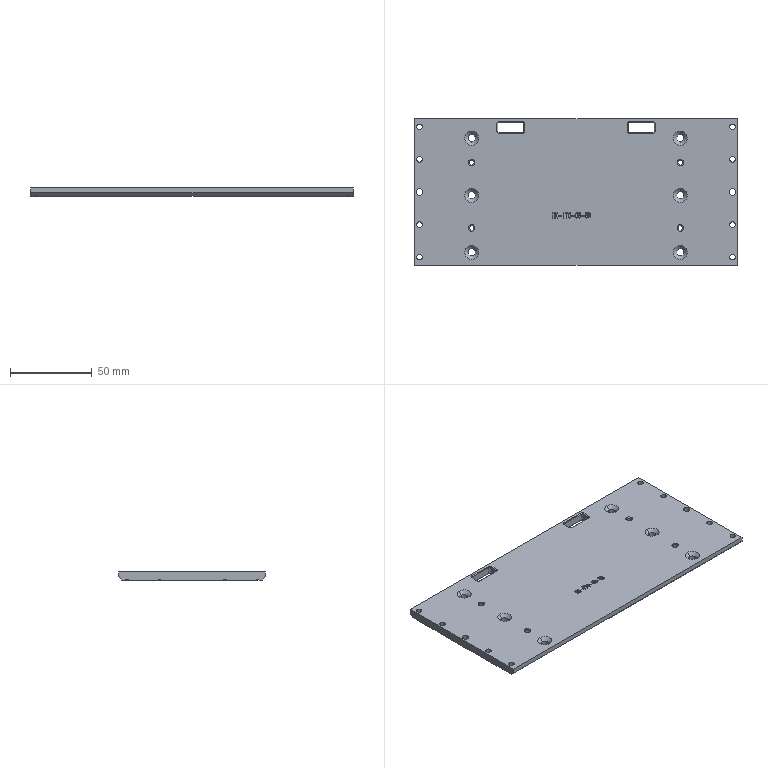NC program | NX | posted with a generic post | part box 198 x 90 x 5 mm
Lines 1 to 1351 of 7160:
N10 G17 G21 G94 G90
(DRILLING , TOOL : D6A45)
N12 T01 M6
N14 G54
N16 G17 G0 G90 X96. Y0. S5000 M3
N18 G43 Z30. H1
N20 G94 G81 G98 Z-2.5 F350. R3.
N22 X-96.
N24 G80
N26 G0 X-96. Y0. Z30.
(DRILLING_COPY , TOOL : D6A45)
N28 X-64. Y-22.
N30 G81 Z-2. F350. R3.
N32 Y18.
N34 X64. Y-22.
N36 Y18.
N38 G80
N40 G0 X64. Y18. Z30.
(DRILLING_COPY_COPY , TOOL : D6A45)
N42 X96. Y40.
N44 G81 Z-2.35 F350. R3.
N46 Y20.
N48 Y-20.
N50 Y-40.
N52 X64. Y-37.
N54 Y-2.
N56 Y33.
N58 X-64.
N60 Y-2.
N62 Y-37.
N64 X-96. Y-40.
N66 Y-20.
N68 Y20.
N70 Y40.
N72 G80
N74 G0 X-96. Y40. Z30.
N76 M5
(DRILLING_COPY_1 , TOOL : 4.5ZT)
N78 T08 M6
N80 G54
N82 G17 G0 G90 X-64. Y-37. S2000 M3
N84 G43 Z30. H8
N86 G94 G83 G98 Z-7.852 F300. Q2. R3.
N88 Y-2.
N90 Y33.
N92 X64.
N94 Y-2.
N96 Y-37.
N98 G80
N100 G0 X64. Y-37. Z30.
N102 M5
(DRILLING_COPY_1_COPY , TOOL : 3.4ZT)
N104 T16 M6
N106 G54
N108 G17 G0 G90 X-96. Y-40. S2000 M3
N110 G43 Z30. H16
N112 G94 G83 G98 Z-6.521 F200. Q2. R3.
N114 Y-20.
N116 Y20.
N118 Y40.
N120 X96.
N122 Y20.
N124 Y-20.
N126 Y-40.
N128 G80
N130 G0 X96. Y-40. Z30.
N132 M5
(ZLEVEL_PROFILE_COPY_1_COPY , TOOL : D10)
N134 T15 M6
N136 G54
N138 G17 G0 G90 X-104.1 Y13.918 S9500 M3
N140 G43 Z30. H15
N142 Z1.5
N144 G94 G1 Y45.554 Z-0.158 F1000.
N146 X-103.766 Y46.898 Z-0.231
N148 X-103.084 Y48.104 Z-0.303
N150 X-102.104 Y49.084 Z-0.376
N152 X-100.898 Y49.766 Z-0.448
N154 X-99.554 Y50.1 Z-0.521
N156 X-99. Z-0.55
N158 X99. F3000.
N160 G2 X104.1 Y45. R5.1
N162 G1 Y-45.
N164 G2 X99. Y-50.1 R5.1
N166 G1 X-99.
N168 G2 X-104.1 Y-45. R5.1
N170 G1 Y45.
N172 G2 X-99. Y50.1 R5.1
N174 G1 X99. Z-0.729
N176 X99.5 Y50.075 Z-0.73
N178 X99.995 Y50.002
N180 X100.48 Y49.88
N182 X100.952 Y49.712 Z-0.731
N184 X101.404 Y49.498
N186 X101.833 Y49.24 Z-0.732
N188 X102.235 Y48.942
N190 X102.606 Y48.606 Z-0.733
N192 X102.942 Y48.235
N194 X103.24 Y47.833 Z-0.734
N196 X103.498 Y47.404
N198 X103.712 Y46.952 Z-0.735
N200 X103.88 Y46.48
N202 X104.002 Y45.995
N204 X104.075 Y45.5 Z-0.736
N206 X104.1 Y45.
N208 X104.103 Y40. Z-0.741
N210 X104.1 Y35. Z-0.745
N212 Y-35. Z-0.809
N214 X104.103 Y-40. Z-0.813
N216 X104.1 Y-45. Z-0.818
N218 X104.075 Y-45.5
N220 X104.002 Y-45.995 Z-0.819
N222 X103.88 Y-46.48
N224 X103.712 Y-46.952 Z-0.82
N226 X103.498 Y-47.404
N228 X103.24 Y-47.833
N230 X102.942 Y-48.235 Z-0.821
N232 X102.606 Y-48.606
N234 X102.235 Y-48.942 Z-0.822
N236 X101.833 Y-49.24
N238 X101.404 Y-49.498 Z-0.823
N240 X100.952 Y-49.712
N242 X100.48 Y-49.88 Z-0.824
N244 X99.995 Y-50.002
N246 X99.5 Y-50.075 Z-0.825
N248 X99. Y-50.1
N250 X-99. Z-1.004
N252 X-99.5 Y-50.075 Z-1.005
N254 X-99.995 Y-50.002
N256 X-100.48 Y-49.88
N258 X-100.952 Y-49.712 Z-1.006
N260 X-101.404 Y-49.498
N262 X-101.833 Y-49.24 Z-1.007
N264 X-102.235 Y-48.942
N266 X-102.606 Y-48.606 Z-1.008
N268 X-102.942 Y-48.235
N270 X-103.24 Y-47.833 Z-1.009
N272 X-103.498 Y-47.404
N274 X-103.712 Y-46.952 Z-1.01
N276 X-103.88 Y-46.48
N278 X-104.002 Y-45.995
N280 X-104.075 Y-45.5 Z-1.011
N282 X-104.1 Y-45.
N284 X-104.103 Y-40. Z-1.016
N286 X-104.1 Y-35. Z-1.02
N288 Y35. Z-1.084
N290 X-104.103 Y40. Z-1.088
N292 X-104.1 Y45. Z-1.093
N294 X-104.075 Y45.5
N296 X-104.002 Y45.995 Z-1.094
N298 X-103.88 Y46.48
N300 X-103.712 Y46.952 Z-1.095
N302 X-103.498 Y47.404
N304 X-103.24 Y47.833
N306 X-102.942 Y48.235 Z-1.096
N308 X-102.606 Y48.606
N310 X-102.235 Y48.942 Z-1.097
N312 X-101.833 Y49.24
N314 X-101.404 Y49.498 Z-1.098
N316 X-100.952 Y49.712
N318 X-100.48 Y49.88 Z-1.099
N320 X-99.995 Y50.002
N322 X-99.5 Y50.075 Z-1.1
N324 X-99. Y50.1
N326 X99. Z-1.279
N328 X99.5 Y50.075 Z-1.28
N330 X99.995 Y50.002
N332 X100.48 Y49.88
N334 X100.952 Y49.712 Z-1.281
N336 X101.404 Y49.498
N338 X101.833 Y49.24 Z-1.282
N340 X102.235 Y48.942
N342 X102.606 Y48.606 Z-1.283
N344 X102.942 Y48.235
N346 X103.24 Y47.833 Z-1.284
N348 X103.498 Y47.404
N350 X103.712 Y46.952 Z-1.285
N352 X103.88 Y46.48
N354 X104.002 Y45.995
N356 X104.075 Y45.5 Z-1.286
N358 X104.1 Y45.
N360 X104.103 Y40. Z-1.291
N362 X104.1 Y35. Z-1.295
N364 Y-35. Z-1.359
N366 X104.103 Y-40. Z-1.363
N368 X104.1 Y-45. Z-1.368
N370 X104.075 Y-45.5
N372 X104.002 Y-45.995 Z-1.369
N374 X103.88 Y-46.48
N376 X103.712 Y-46.952 Z-1.37
N378 X103.498 Y-47.404
N380 X103.24 Y-47.833
N382 X102.942 Y-48.235 Z-1.371
N384 X102.606 Y-48.606
N386 X102.235 Y-48.942 Z-1.372
N388 X101.833 Y-49.24
N390 X101.404 Y-49.498 Z-1.373
N392 X100.952 Y-49.712
N394 X100.48 Y-49.88 Z-1.374
N396 X99.995 Y-50.002
N398 X99.5 Y-50.075 Z-1.375
N400 X99. Y-50.1
N402 X-99. Z-1.554
N404 X-99.5 Y-50.075 Z-1.555
N406 X-99.995 Y-50.002
N408 X-100.48 Y-49.88
N410 X-100.952 Y-49.712 Z-1.556
N412 X-101.404 Y-49.498
N414 X-101.833 Y-49.24 Z-1.557
N416 X-102.235 Y-48.942
N418 X-102.606 Y-48.606 Z-1.558
N420 X-102.942 Y-48.235
N422 X-103.24 Y-47.833 Z-1.559
N424 X-103.498 Y-47.404
N426 X-103.712 Y-46.952 Z-1.56
N428 X-103.88 Y-46.48
N430 X-104.002 Y-45.995
N432 X-104.075 Y-45.5 Z-1.561
N434 X-104.1 Y-45.
N436 X-104.103 Y-40. Z-1.566
N438 X-104.1 Y-35. Z-1.57
N440 Y35. Z-1.634
N442 X-104.103 Y40. Z-1.638
N444 X-104.1 Y45. Z-1.643
N446 X-104.075 Y45.5
N448 X-104.002 Y45.995 Z-1.644
N450 X-103.88 Y46.48
N452 X-103.712 Y46.952 Z-1.645
N454 X-103.498 Y47.404
N456 X-103.24 Y47.833
N458 X-102.942 Y48.235 Z-1.646
N460 X-102.606 Y48.606
N462 X-102.235 Y48.942 Z-1.647
N464 X-101.833 Y49.24
N466 X-101.404 Y49.498 Z-1.648
N468 X-100.952 Y49.712
N470 X-100.48 Y49.88 Z-1.649
N472 X-99.995 Y50.002
N474 X-99.5 Y50.075 Z-1.65
N476 X-99. Y50.1
N478 X99. Z-1.829
N480 X99.5 Y50.075 Z-1.83
N482 X99.995 Y50.002
N484 X100.48 Y49.88
N486 X100.952 Y49.712 Z-1.831
N488 X101.404 Y49.498
N490 X101.833 Y49.24 Z-1.832
N492 X102.235 Y48.942
N494 X102.606 Y48.606 Z-1.833
N496 X102.942 Y48.235
N498 X103.24 Y47.833 Z-1.834
N500 X103.498 Y47.404
N502 X103.712 Y46.952 Z-1.835
N504 X103.88 Y46.48
N506 X104.002 Y45.995
N508 X104.075 Y45.5 Z-1.836
N510 X104.1 Y45.
N512 X104.103 Y40. Z-1.841
N514 X104.1 Y35. Z-1.845
N516 Y-35. Z-1.909
N518 X104.103 Y-40. Z-1.913
N520 X104.1 Y-45. Z-1.918
N522 X104.075 Y-45.5
N524 X104.002 Y-45.995 Z-1.919
N526 X103.88 Y-46.48
N528 X103.712 Y-46.952 Z-1.92
N530 X103.498 Y-47.404
N532 X103.24 Y-47.833
N534 X102.942 Y-48.235 Z-1.921
N536 X102.606 Y-48.606
N538 X102.235 Y-48.942 Z-1.922
N540 X101.833 Y-49.24
N542 X101.404 Y-49.498 Z-1.923
N544 X100.952 Y-49.712
N546 X100.48 Y-49.88 Z-1.924
N548 X99.995 Y-50.002
N550 X99.5 Y-50.075 Z-1.925
N552 X99. Y-50.1
N554 X-99. Z-2.104
N556 X-99.5 Y-50.075 Z-2.105
N558 X-99.995 Y-50.002
N560 X-100.48 Y-49.88
N562 X-100.952 Y-49.712 Z-2.106
N564 X-101.404 Y-49.498
N566 X-101.833 Y-49.24 Z-2.107
N568 X-102.235 Y-48.942
N570 X-102.606 Y-48.606 Z-2.108
N572 X-102.942 Y-48.235
N574 X-103.24 Y-47.833 Z-2.109
N576 X-103.498 Y-47.404
N578 X-103.712 Y-46.952 Z-2.11
N580 X-103.88 Y-46.48
N582 X-104.002 Y-45.995
N584 X-104.075 Y-45.5 Z-2.111
N586 X-104.1 Y-45.
N588 X-104.103 Y-40. Z-2.116
N590 X-104.1 Y-35. Z-2.12
N592 Y35. Z-2.184
N594 X-104.103 Y40. Z-2.188
N596 X-104.1 Y45. Z-2.193
N598 X-104.075 Y45.5
N600 X-104.002 Y45.995 Z-2.194
N602 X-103.88 Y46.48
N604 X-103.712 Y46.952 Z-2.195
N606 X-103.498 Y47.404
N608 X-103.24 Y47.833
N610 X-102.942 Y48.235 Z-2.196
N612 X-102.606 Y48.606
N614 X-102.235 Y48.942 Z-2.197
N616 X-101.833 Y49.24
N618 X-101.404 Y49.498 Z-2.198
N620 X-100.952 Y49.712
N622 X-100.48 Y49.88 Z-2.199
N624 X-99.995 Y50.002
N626 X-99.5 Y50.075 Z-2.2
N628 X-99. Y50.1
N630 X99. Z-2.379
N632 X99.5 Y50.075 Z-2.38
N634 X99.995 Y50.002
N636 X100.48 Y49.88
N638 X100.952 Y49.712 Z-2.381
N640 X101.404 Y49.498
N642 X101.833 Y49.24 Z-2.382
N644 X102.235 Y48.942
N646 X102.606 Y48.606 Z-2.383
N648 X102.942 Y48.235
N650 X103.24 Y47.833 Z-2.384
N652 X103.498 Y47.404
N654 X103.712 Y46.952 Z-2.385
N656 X103.88 Y46.48
N658 X104.002 Y45.995
N660 X104.075 Y45.5 Z-2.386
N662 X104.1 Y45.
N664 X104.103 Y40. Z-2.391
N666 X104.1 Y35. Z-2.395
N668 Y-35. Z-2.459
N670 X104.103 Y-40. Z-2.463
N672 X104.1 Y-45. Z-2.468
N674 X104.075 Y-45.5
N676 X104.002 Y-45.995 Z-2.469
N678 X103.88 Y-46.48
N680 X103.712 Y-46.952 Z-2.47
N682 X103.498 Y-47.404
N684 X103.24 Y-47.833
N686 X102.942 Y-48.235 Z-2.471
N688 X102.606 Y-48.606
N690 X102.235 Y-48.942 Z-2.472
N692 X101.833 Y-49.24
N694 X101.404 Y-49.498 Z-2.473
N696 X100.952 Y-49.712
N698 X100.48 Y-49.88 Z-2.474
N700 X99.995 Y-50.002
N702 X99.5 Y-50.075 Z-2.475
N704 X99. Y-50.1
N706 X-99. Z-2.654
N708 X-99.5 Y-50.075 Z-2.655
N710 X-99.995 Y-50.002
N712 X-100.48 Y-49.88
N714 X-100.952 Y-49.712 Z-2.656
N716 X-101.404 Y-49.498
N718 X-101.833 Y-49.24 Z-2.657
N720 X-102.235 Y-48.942
N722 X-102.606 Y-48.606 Z-2.658
N724 X-102.942 Y-48.235
N726 X-103.24 Y-47.833 Z-2.659
N728 X-103.498 Y-47.404
N730 X-103.712 Y-46.952 Z-2.66
N732 X-103.88 Y-46.48
N734 X-104.002 Y-45.995
N736 X-104.075 Y-45.5 Z-2.661
N738 X-104.1 Y-45.
N740 X-104.103 Y-40. Z-2.666
N742 X-104.1 Y-35. Z-2.67
N744 Y35. Z-2.734
N746 X-104.103 Y40. Z-2.738
N748 X-104.1 Y45. Z-2.743
N750 X-104.075 Y45.5
N752 X-104.002 Y45.995 Z-2.744
N754 X-103.88 Y46.48
N756 X-103.712 Y46.952 Z-2.745
N758 X-103.498 Y47.404
N760 X-103.24 Y47.833
N762 X-102.942 Y48.235 Z-2.746
N764 X-102.606 Y48.606
N766 X-102.235 Y48.942 Z-2.747
N768 X-101.833 Y49.24
N770 X-101.404 Y49.498 Z-2.748
N772 X-100.952 Y49.712
N774 X-100.48 Y49.88 Z-2.749
N776 X-99.995 Y50.002
N778 X-99.5 Y50.075 Z-2.75
N780 X-99. Y50.1
N782 X99. Z-2.929
N784 X99.5 Y50.075 Z-2.93
N786 X99.995 Y50.002
N788 X100.48 Y49.88
N790 X100.952 Y49.712 Z-2.931
N792 X101.404 Y49.498
N794 X101.833 Y49.24 Z-2.932
N796 X102.235 Y48.942
N798 X102.606 Y48.606 Z-2.933
N800 X102.942 Y48.235
N802 X103.24 Y47.833 Z-2.934
N804 X103.498 Y47.404
N806 X103.712 Y46.952 Z-2.935
N808 X103.88 Y46.48
N810 X104.002 Y45.995
N812 X104.075 Y45.5 Z-2.936
N814 X104.1 Y45.
N816 X104.103 Y40. Z-2.941
N818 X104.1 Y35. Z-2.945
N820 Y-35. Z-3.009
N822 X104.103 Y-40. Z-3.013
N824 X104.1 Y-45. Z-3.018
N826 X104.075 Y-45.5
N828 X104.002 Y-45.995 Z-3.019
N830 X103.88 Y-46.48
N832 X103.712 Y-46.952 Z-3.02
N834 X103.498 Y-47.404
N836 X103.24 Y-47.833
N838 X102.942 Y-48.235 Z-3.021
N840 X102.606 Y-48.606
N842 X102.235 Y-48.942 Z-3.022
N844 X101.833 Y-49.24
N846 X101.404 Y-49.498 Z-3.023
N848 X100.952 Y-49.712
N850 X100.48 Y-49.88 Z-3.024
N852 X99.995 Y-50.002
N854 X99.5 Y-50.075 Z-3.025
N856 X99. Y-50.1
N858 X-99. Z-3.204
N860 X-99.5 Y-50.075 Z-3.205
N862 X-99.995 Y-50.002
N864 X-100.48 Y-49.88
N866 X-100.952 Y-49.712 Z-3.206
N868 X-101.404 Y-49.498
N870 X-101.833 Y-49.24 Z-3.207
N872 X-102.235 Y-48.942
N874 X-102.606 Y-48.606 Z-3.208
N876 X-102.942 Y-48.235
N878 X-103.24 Y-47.833 Z-3.209
N880 X-103.498 Y-47.404
N882 X-103.712 Y-46.952 Z-3.21
N884 X-103.88 Y-46.48
N886 X-104.002 Y-45.995
N888 X-104.075 Y-45.5 Z-3.211
N890 X-104.1 Y-45.
N892 X-104.103 Y-40. Z-3.216
N894 X-104.1 Y-35. Z-3.22
N896 Y35. Z-3.284
N898 X-104.103 Y40. Z-3.288
N900 X-104.1 Y45. Z-3.293
N902 X-104.075 Y45.5
N904 X-104.002 Y45.995 Z-3.294
N906 X-103.88 Y46.48
N908 X-103.712 Y46.952 Z-3.295
N910 X-103.498 Y47.404
N912 X-103.24 Y47.833
N914 X-102.942 Y48.235 Z-3.296
N916 X-102.606 Y48.606
N918 X-102.235 Y48.942 Z-3.297
N920 X-101.833 Y49.24
N922 X-101.404 Y49.498 Z-3.298
N924 X-100.952 Y49.712
N926 X-100.48 Y49.88 Z-3.299
N928 X-99.995 Y50.002
N930 X-99.5 Y50.075 Z-3.3
N932 X-99. Y50.1
N934 X99. Z-3.479
N936 X99.5 Y50.075 Z-3.48
N938 X99.995 Y50.002
N940 X100.48 Y49.88
N942 X100.952 Y49.712 Z-3.481
N944 X101.404 Y49.498
N946 X101.833 Y49.24 Z-3.482
N948 X102.235 Y48.942
N950 X102.606 Y48.606 Z-3.483
N952 X102.942 Y48.235
N954 X103.24 Y47.833 Z-3.484
N956 X103.498 Y47.404
N958 X103.712 Y46.952 Z-3.485
N960 X103.88 Y46.48
N962 X104.002 Y45.995
N964 X104.075 Y45.5 Z-3.486
N966 X104.1 Y45.
N968 X104.103 Y40. Z-3.491
N970 X104.1 Y35. Z-3.495
N972 Y-35. Z-3.559
N974 X104.103 Y-40. Z-3.563
N976 X104.1 Y-45. Z-3.568
N978 X104.075 Y-45.5
N980 X104.002 Y-45.995 Z-3.569
N982 X103.88 Y-46.48
N984 X103.712 Y-46.952 Z-3.57
N986 X103.498 Y-47.404
N988 X103.24 Y-47.833
N990 X102.942 Y-48.235 Z-3.571
N992 X102.606 Y-48.606
N994 X102.235 Y-48.942 Z-3.572
N996 X101.833 Y-49.24
N998 X101.404 Y-49.498 Z-3.573
N1000 X100.952 Y-49.712
N1002 X100.48 Y-49.88 Z-3.574
N1004 X99.995 Y-50.002
N1006 X99.5 Y-50.075 Z-3.575
N1008 X99. Y-50.1
N1010 X-99. Z-3.754
N1012 X-99.5 Y-50.075 Z-3.755
N1014 X-99.995 Y-50.002
N1016 X-100.48 Y-49.88
N1018 X-100.952 Y-49.712 Z-3.756
N1020 X-101.404 Y-49.498
N1022 X-101.833 Y-49.24 Z-3.757
N1024 X-102.235 Y-48.942
N1026 X-102.606 Y-48.606 Z-3.758
N1028 X-102.942 Y-48.235
N1030 X-103.24 Y-47.833 Z-3.759
N1032 X-103.498 Y-47.404
N1034 X-103.712 Y-46.952 Z-3.76
N1036 X-103.88 Y-46.48
N1038 X-104.002 Y-45.995
N1040 X-104.075 Y-45.5 Z-3.761
N1042 X-104.1 Y-45.
N1044 X-104.103 Y-40. Z-3.766
N1046 X-104.1 Y-35. Z-3.77
N1048 Y35. Z-3.834
N1050 X-104.103 Y40. Z-3.838
N1052 X-104.1 Y45. Z-3.843
N1054 X-104.075 Y45.5
N1056 X-104.002 Y45.995 Z-3.844
N1058 X-103.88 Y46.48
N1060 X-103.712 Y46.952 Z-3.845
N1062 X-103.498 Y47.404
N1064 X-103.24 Y47.833
N1066 X-102.942 Y48.235 Z-3.846
N1068 X-102.606 Y48.606
N1070 X-102.235 Y48.942 Z-3.847
N1072 X-101.833 Y49.24
N1074 X-101.404 Y49.498 Z-3.848
N1076 X-100.952 Y49.712
N1078 X-100.48 Y49.88 Z-3.849
N1080 X-99.995 Y50.002
N1082 X-99.5 Y50.075 Z-3.85
N1084 X-99. Y50.1
N1086 X99. Z-4.029
N1088 X99.5 Y50.075 Z-4.03
N1090 X99.995 Y50.002
N1092 X100.48 Y49.88
N1094 X100.952 Y49.712 Z-4.031
N1096 X101.404 Y49.498
N1098 X101.833 Y49.24 Z-4.032
N1100 X102.235 Y48.942
N1102 X102.606 Y48.606 Z-4.033
N1104 X102.942 Y48.235
N1106 X103.24 Y47.833 Z-4.034
N1108 X103.498 Y47.404
N1110 X103.712 Y46.952 Z-4.035
N1112 X103.88 Y46.48
N1114 X104.002 Y45.995
N1116 X104.075 Y45.5 Z-4.036
N1118 X104.1 Y45.
N1120 X104.103 Y40. Z-4.041
N1122 X104.1 Y35. Z-4.045
N1124 Y-35. Z-4.109
N1126 X104.103 Y-40. Z-4.113
N1128 X104.1 Y-45. Z-4.118
N1130 X104.075 Y-45.5
N1132 X104.002 Y-45.995 Z-4.119
N1134 X103.88 Y-46.48
N1136 X103.712 Y-46.952 Z-4.12
N1138 X103.498 Y-47.404
N1140 X103.24 Y-47.833
N1142 X102.942 Y-48.235 Z-4.121
N1144 X102.606 Y-48.606
N1146 X102.235 Y-48.942 Z-4.122
N1148 X101.833 Y-49.24
N1150 X101.404 Y-49.498 Z-4.123
N1152 X100.952 Y-49.712
N1154 X100.48 Y-49.88 Z-4.124
N1156 X99.995 Y-50.002
N1158 X99.5 Y-50.075 Z-4.125
N1160 X99. Y-50.1
N1162 X-99. Z-4.304
N1164 X-99.5 Y-50.075 Z-4.305
N1166 X-99.995 Y-50.002
N1168 X-100.48 Y-49.88
N1170 X-100.952 Y-49.712 Z-4.306
N1172 X-101.404 Y-49.498
N1174 X-101.833 Y-49.24 Z-4.307
N1176 X-102.235 Y-48.942
N1178 X-102.606 Y-48.606 Z-4.308
N1180 X-102.942 Y-48.235
N1182 X-103.24 Y-47.833 Z-4.309
N1184 X-103.498 Y-47.404
N1186 X-103.712 Y-46.952 Z-4.31
N1188 X-103.88 Y-46.48
N1190 X-104.002 Y-45.995
N1192 X-104.075 Y-45.5 Z-4.311
N1194 X-104.1 Y-45.
N1196 X-104.103 Y-40. Z-4.316
N1198 X-104.1 Y-35. Z-4.32
N1200 Y35. Z-4.384
N1202 X-104.103 Y40. Z-4.388
N1204 X-104.1 Y45. Z-4.393
N1206 X-104.075 Y45.5
N1208 X-104.002 Y45.995 Z-4.394
N1210 X-103.88 Y46.48
N1212 X-103.712 Y46.952 Z-4.395
N1214 X-103.498 Y47.404
N1216 X-103.24 Y47.833
N1218 X-102.942 Y48.235 Z-4.396
N1220 X-102.606 Y48.606
N1222 X-102.235 Y48.942 Z-4.397
N1224 X-101.833 Y49.24
N1226 X-101.404 Y49.498 Z-4.398
N1228 X-100.952 Y49.712
N1230 X-100.48 Y49.88 Z-4.399
N1232 X-99.995 Y50.002
N1234 X-99.5 Y50.075 Z-4.4
N1236 X-99. Y50.1
N1238 X99.
N1240 G2 X104.1 Y45. R5.1
N1242 G1 Y-45.
N1244 G2 X99. Y-50.1 R5.1
N1246 G1 X-99.
N1248 G2 X-104.1 Y-45. R5.1
N1250 G1 Y45.
N1252 G2 X-99. Y50.1 R5.1
N1254 G1 Z-2.9
N1256 G0 Z30.
(FLOOR_WALL , TOOL : D10)
N1258 X75.1 Y-14.822
N1260 Z1.5
N1262 G1 Y-26.5 Z0.888 F1000.
N1264 Y-26.734 Z0.876
N1266 X75.342 Y-27.158 Z0.85
N1268 X75.766 Y-27.4 Z0.825
N1270 X82.234 Z0.486
N1272 X82.658 Y-27.158 Z0.46
N1274 X82.9 Y-26.734 Z0.434
N1276 Y-26.5 Z0.422
N1278 Y0. Z-0.967
N1280 Y26.5 F3000.
N1282 G3 X82. Y27.4 R0.9
N1284 G1 X76.
N1286 G3 X75.1 Y26.5 R0.9
N1288 G1 Y-26.5
N1290 G3 X76. Y-27.4 R0.9
N1292 G1 X82.
N1294 G3 X82.9 Y-26.5 R0.9
N1296 G1 Y0.
N1298 Z0.533
N1300 G0 X75.1 Y-14.822
N1302 G1 Y-26.5 Z-0.079 F1000.
N1304 Y-26.734 Z-0.091
N1306 X75.342 Y-27.158 Z-0.117
N1308 X75.766 Y-27.4 Z-0.142
N1310 X82.234 Z-0.481
N1312 X82.658 Y-27.158 Z-0.507
N1314 X82.9 Y-26.734 Z-0.532
N1316 Y-26.5 Z-0.545
N1318 Y0. Z-1.933
N1320 Y26.5 F3000.
N1322 G3 X82. Y27.4 R0.9
N1324 G1 X76.
N1326 G3 X75.1 Y26.5 R0.9
N1328 G1 Y-26.5
N1330 G3 X76. Y-27.4 R0.9
N1332 G1 X82.
N1334 G3 X82.9 Y-26.5 R0.9
N1336 G1 Y0.
N1338 Z-0.433
N1340 G0 X75.1 Y-14.822
N1342 G1 Y-26.5 Z-1.045 F1000.
N1344 Y-26.734 Z-1.058
N1346 X75.342 Y-27.158 Z-1.083
N1348 X75.766 Y-27.4 Z-1.109
N1350 X82.234 Z-1.448
N1352 X82.658 Y-27.158 Z-1.473
N1354 X82.9 Y-26.734 Z-1.499
N1356 Y-26.5 Z-1.511
N1358 Y0. Z-2.9
N1360 Y26.5 F3000.
N1362 G3 X82. Y27.4 R0.9
N1364 G1 X76.
N1366 G3 X75.1 Y26.5 R0.9
N1368 G1 Y-26.5
N1370 G3 X76. Y-27.4 R0.9
N1372 G1 X82.
N1374 G3 X82.9 Y-26.5 R0.9
N1376 G1 Y0.
N1378 Z-1.4
N1380 G0 Z30.
N1382 X-31.9 Y0.267
N1384 Z1.5
N1386 G1 Y-6.4 Z1.151 F1000.
N1388 X-29.1 Z1.004
N1390 Y6.4 Z0.333
N1392 X-31.9 Z0.186
N1394 Y-6.4 Z-0.485
N1396 X-29.1 Z-0.631
N1398 Y0. Z-0.967
N1400 Y6.4 F3000.
N1402 X-31.9
N1404 Y-6.4
N1406 X-29.1
N1408 Y0.
N1410 X-22.1
N1412 Y13.4
N1414 X-38.9
N1416 Y-13.4
N1418 X-22.1
N1420 Y0.
N1422 X-15.1
N1424 Y20.4
N1426 X-45.9
N1428 Y-20.4
N1430 X-15.1
N1432 Y0.
N1434 X-8.1
N1436 Y26.5
N1438 G3 X-9. Y27.4 R0.9
N1440 G1 X-52.
N1442 G3 X-52.9 Y26.5 R0.9
N1444 G1 Y-26.5
N1446 G3 X-52. Y-27.4 R0.9
N1448 G1 X-9.
N1450 G3 X-8.1 Y-26.5 R0.9
N1452 G1 Y0.
N1454 Z0.533
N1456 G0 X-31.9 Y0.267
N1458 G1 Y-6.4 Z0.184 F1000.
N1460 X-29.1 Z0.037
N1462 Y6.4 Z-0.634
N1464 X-31.9 Z-0.78
N1466 Y-6.4 Z-1.451
N1468 X-29.1 Z-1.598
N1470 Y0. Z-1.933
N1472 Y6.4 F3000.
N1474 X-31.9
N1476 Y-6.4
N1478 X-29.1
N1480 Y0.
N1482 X-22.1
N1484 Y13.4
N1486 X-38.9
N1488 Y-13.4
N1490 X-22.1
N1492 Y0.
N1494 X-15.1
N1496 Y20.4
N1498 X-45.9
N1500 Y-20.4
N1502 X-15.1
N1504 Y0.
N1506 X-8.1
N1508 Y26.5
N1510 G3 X-9. Y27.4 R0.9
N1512 G1 X-52.
N1514 G3 X-52.9 Y26.5 R0.9
N1516 G1 Y-26.5
N1518 G3 X-52. Y-27.4 R0.9
N1520 G1 X-9.
N1522 G3 X-8.1 Y-26.5 R0.9
N1524 G1 Y0.
N1526 Z-0.433
N1528 G0 X-31.9 Y0.267
N1530 G1 Y-6.4 Z-0.783 F1000.
N1532 X-29.1 Z-0.929
N1534 Y6.4 Z-1.6
N1536 X-31.9 Z-1.747
N1538 Y-6.4 Z-2.418
N1540 X-29.1 Z-2.565
N1542 Y0. Z-2.9
N1544 Y6.4 F3000.
N1546 X-31.9
N1548 Y-6.4
N1550 X-29.1
N1552 Y0.
N1554 X-22.1
N1556 Y13.4
N1558 X-38.9
N1560 Y-13.4
N1562 X-22.1
N1564 Y0.
N1566 X-15.1
N1568 Y20.4
N1570 X-45.9
N1572 Y-20.4
N1574 X-15.1
N1576 Y0.
N1578 X-8.1
N1580 Y26.5
N1582 G3 X-9. Y27.4 R0.9
N1584 G1 X-52.
N1586 G3 X-52.9 Y26.5 R0.9
N1588 G1 Y-26.5
N1590 G3 X-52. Y-27.4 R0.9
N1592 G1 X-9.
N1594 G3 X-8.1 Y-26.5 R0.9
N1596 G1 Y0.
N1598 Z-1.4
N1600 G0 Z30.
N1602 X31.9 Y-0.267
N1604 Z1.5
N1606 G1 Y6.4 Z1.151 F1000.
N1608 X29.1 Z1.004
N1610 Y-6.4 Z0.333
N1612 X31.9 Z0.186
N1614 Y6.4 Z-0.485
N1616 X29.1 Z-0.631
N1618 Y0. Z-0.967
N1620 Y-6.4 F3000.
N1622 X31.9
N1624 Y6.4
N1626 X29.1
N1628 Y0.
N1630 X22.1
N1632 Y-13.4
N1634 X38.9
N1636 Y13.4
N1638 X22.1
N1640 Y0.
N1642 X15.1
N1644 Y-20.4
N1646 X45.9
N1648 Y20.4
N1650 X15.1
N1652 Y0.
N1654 X8.1
N1656 Y-26.5
N1658 G3 X9. Y-27.4 R0.9
N1660 G1 X52.
N1662 G3 X52.9 Y-26.5 R0.9
N1664 G1 Y26.5
N1666 G3 X52. Y27.4 R0.9
N1668 G1 X9.
N1670 G3 X8.1 Y26.5 R0.9
N1672 G1 Y0.
N1674 Z0.533
N1676 G0 X31.9 Y-0.267
N1678 G1 Y6.4 Z0.184 F1000.
N1680 X29.1 Z0.037
N1682 Y-6.4 Z-0.634
N1684 X31.9 Z-0.78
N1686 Y6.4 Z-1.451
N1688 X29.1 Z-1.598
N1690 Y0. Z-1.933
N1692 Y-6.4 F3000.
N1694 X31.9
N1696 Y6.4
N1698 X29.1
N1700 Y0.
N1702 X22.1
N1704 Y-13.4
N1706 X38.9
N1708 Y13.4
N1710 X22.1
N1712 Y0.
N1714 X15.1
N1716 Y-20.4
N1718 X45.9
N1720 Y20.4
N1722 X15.1
N1724 Y0.
N1726 X8.1
N1728 Y-26.5
N1730 G3 X9. Y-27.4 R0.9
N1732 G1 X52.
N1734 G3 X52.9 Y-26.5 R0.9
N1736 G1 Y26.5
N1738 G3 X52. Y27.4 R0.9
N1740 G1 X9.
N1742 G3 X8.1 Y26.5 R0.9
N1744 G1 Y0.
N1746 Z-0.433
N1748 G0 X31.9 Y-0.267
N1750 G1 Y6.4 Z-0.783 F1000.
N1752 X29.1 Z-0.929
N1754 Y-6.4 Z-1.6
N1756 X31.9 Z-1.747
N1758 Y6.4 Z-2.418
N1760 X29.1 Z-2.565
N1762 Y0. Z-2.9
N1764 Y-6.4 F3000.
N1766 X31.9
N1768 Y6.4
N1770 X29.1
N1772 Y0.
N1774 X22.1
N1776 Y-13.4
N1778 X38.9
N1780 Y13.4
N1782 X22.1
N1784 Y0.
N1786 X15.1
N1788 Y-20.4
N1790 X45.9
N1792 Y20.4
N1794 X15.1
N1796 Y0.
N1798 X8.1
N1800 Y-26.5
N1802 G3 X9. Y-27.4 R0.9
N1804 G1 X52.
N1806 G3 X52.9 Y-26.5 R0.9
N1808 G1 Y26.5
N1810 G3 X52. Y27.4 R0.9
N1812 G1 X9.
N1814 G3 X8.1 Y26.5 R0.9
N1816 G1 Y0.
N1818 Z-1.4
N1820 G0 Z30.
N1822 X-75.1 Y14.822
N1824 Z1.5
N1826 G1 Y26.5 Z0.888 F1000.
N1828 Y26.734 Z0.876
N1830 X-75.342 Y27.158 Z0.85
N1832 X-75.766 Y27.4 Z0.825
N1834 X-82.234 Z0.486
N1836 X-82.658 Y27.158 Z0.46
N1838 X-82.9 Y26.734 Z0.434
N1840 Y0. Z-0.967
N1842 Y-26.5 F3000.
N1844 G3 X-82. Y-27.4 R0.9
N1846 G1 X-76.
N1848 G3 X-75.1 Y-26.5 R0.9
N1850 G1 Y26.5
N1852 G3 X-76. Y27.4 R0.9
N1854 G1 X-82.
N1856 G3 X-82.9 Y26.5 R0.9
N1858 G1 Y0.
N1860 Z0.533
N1862 G0 X-75.1 Y14.822
N1864 G1 Y26.5 Z-0.079 F1000.
N1866 Y26.734 Z-0.091
N1868 X-75.342 Y27.158 Z-0.117
N1870 X-75.766 Y27.4 Z-0.142
N1872 X-82.234 Z-0.481
N1874 X-82.658 Y27.158 Z-0.507
N1876 X-82.9 Y26.734 Z-0.532
N1878 Y0. Z-1.933
N1880 Y-26.5 F3000.
N1882 G3 X-82. Y-27.4 R0.9
N1884 G1 X-76.
N1886 G3 X-75.1 Y-26.5 R0.9
N1888 G1 Y26.5
N1890 G3 X-76. Y27.4 R0.9
N1892 G1 X-82.
N1894 G3 X-82.9 Y26.5 R0.9
N1896 G1 Y0.
N1898 Z-0.433
N1900 G0 X-75.1 Y14.822
N1902 G1 Y26.5 Z-1.045 F1000.
N1904 Y26.734 Z-1.058
N1906 X-75.342 Y27.158 Z-1.083
N1908 X-75.766 Y27.4 Z-1.109
N1910 X-82.234 Z-1.448
N1912 X-82.658 Y27.158 Z-1.473
N1914 X-82.9 Y26.734 Z-1.499
N1916 Y0. Z-2.9
N1918 Y-26.5 F3000.
N1920 G3 X-82. Y-27.4 R0.9
N1922 G1 X-76.
N1924 G3 X-75.1 Y-26.5 R0.9
N1926 G1 Y26.5
N1928 G3 X-76. Y27.4 R0.9
N1930 G1 X-82.
N1932 G3 X-82.9 Y26.5 R0.9
N1934 G1 Y0.
N1936 Z-1.4
N1938 G0 Z30.
N1940 M5
(FLOOR_WALL_COPY , TOOL : D10JING)
N1942 T14 M6
N1944 G54
N1946 G17 G0 G90 X-82. Y0.866 S9500 M3
N1948 G43 Z30. H14
N1950 Z-2.
N1952 G94 G1 Z-3. F1000.
N1954 G3 X-82.5 Y0. R1.
N1956 G1 Y26.5 F1500.
N1958 G2 X-82. Y27. R0.5
N1960 G1 X-76.
N1962 G2 X-75.5 Y26.5 R0.5
N1964 G1 Y-26.5
N1966 G2 X-76. Y-27. R0.5
N1968 G1 X-82.
N1970 G2 X-82.5 Y-26.5 R0.5
N1972 G1 Y0.
N1974 Y0.866
N1976 G3 X-83. Y0. R1. F1000.
N1978 G1 Y-26.5 F1500.
N1980 G3 X-82. Y-27.5 R1.
N1982 G1 X-76.
N1984 G3 X-75. Y-26.5 R1.
N1986 G1 Y26.5
N1988 G3 X-76. Y27.5 R1.
N1990 G1 X-82.
N1992 G3 X-83. Y26.5 R1.
N1994 G1 Y0.
N1996 G3 X-82.5 Y-0.866 R1.
N1998 G1 X-81.5 Y-1.443
N2000 Z-2.
N2002 G0 Z30.
N2004 X9. Y0.866
N2006 Z-2.
N2008 G1 Z-3. F1000.
N2010 G3 X8.5 Y0. R1.
N2012 G1 Y26.5 F1500.
N2014 G2 X9. Y27. R0.5
N2016 G1 X52.
N2018 G2 X52.5 Y26.5 R0.5
N2020 G1 Y-26.5
N2022 G2 X52. Y-27. R0.5
N2024 G1 X9.
N2026 G2 X8.5 Y-26.5 R0.5
N2028 G1 Y0.
N2030 X13.5
N2032 Y22.
N2034 X47.5
N2036 Y-22.
N2038 X13.5
N2040 Y0.
N2042 X18.5
N2044 Y17.
N2046 X42.5
N2048 Y-17.
N2050 X18.5
N2052 Y0.
N2054 X23.5
N2056 Y12.
N2058 X37.5
N2060 Y-12.
N2062 X23.5
N2064 Y0.
N2066 X28.5
N2068 Y7.
N2070 X32.5
N2072 Y-7.
N2074 X28.5
N2076 Y0.
N2078 G3 X28. Y0.866 R1.
N2080 G1 Z-2.
N2082 G0 Z30.
N2084 X10. Y1.732
N2086 Z-2.
N2088 G1 Z-3. F1000.
N2090 X8.5 Y0.866
N2092 G3 X8. Y0. R1.
N2094 G1 Y-26.5 F1500.
N2096 G3 X9. Y-27.5 R1.
N2098 G1 X52.
N2100 G3 X53. Y-26.5 R1.
N2102 G1 Y26.5
N2104 G3 X52. Y27.5 R1.
N2106 G1 X9.
N2108 G3 X8. Y26.5 R1.
N2110 G1 Y0.
N2112 G3 X8.5 Y-0.866 R1.
N2114 G1 X9.5 Y-1.443
N2116 Z-2.
N2118 G0 Z30.
N2120 X-9. Y-0.866
N2122 Z-2.
N2124 G1 Z-3. F1000.
N2126 G3 X-8.5 Y0. R1.
N2128 G1 Y-26.5 F1500.
N2130 G2 X-9. Y-27. R0.5
N2132 G1 X-52.
N2134 G2 X-52.5 Y-26.5 R0.5
N2136 G1 Y26.5
N2138 G2 X-52. Y27. R0.5
N2140 G1 X-9.
N2142 G2 X-8.5 Y26.5 R0.5
N2144 G1 Y0.
N2146 X-13.5
N2148 Y-22.
N2150 X-47.5
N2152 Y22.
N2154 X-13.5
N2156 Y0.
N2158 X-18.5
N2160 Y-17.
N2162 X-42.5
N2164 Y17.
N2166 X-18.5
N2168 Y0.
N2170 X-23.5
N2172 Y-12.
N2174 X-37.5
N2176 Y12.
N2178 X-23.5
N2180 Y0.
N2182 X-28.5
N2184 Y-7.
N2186 X-32.5
N2188 Y7.
N2190 X-28.5
N2192 Y0.
N2194 G3 X-28. Y-0.866 R1.
N2196 G1 Z-2.
N2198 G0 Z30.
N2200 X-10. Y-1.732
N2202 Z-2.
N2204 G1 Z-3. F1000.
N2206 X-8.5 Y-0.866
N2208 G3 X-8. Y0. R1.
N2210 G1 Y26.5 F1500.
N2212 G3 X-9. Y27.5 R1.
N2214 G1 X-52.
N2216 G3 X-53. Y26.5 R1.
N2218 G1 Y-26.5
N2220 G3 X-52. Y-27.5 R1.
N2222 G1 X-9.
N2224 G3 X-8. Y-26.5 R1.
N2226 G1 Y0.
N2228 G3 X-8.5 Y0.866 R1.
N2230 G1 X-9.5 Y1.443
N2232 Z-2.
N2234 G0 Z30.
N2236 X82. Y-0.866
N2238 Z-2.
N2240 G1 Z-3. F1000.
N2242 G3 X82.5 Y0. R1.
N2244 G1 Y-26.5 F1500.
N2246 G2 X82. Y-27. R0.5
N2248 G1 X76.
N2250 G2 X75.5 Y-26.5 R0.5
N2252 G1 Y26.5
N2254 G2 X76. Y27. R0.5
N2256 G1 X82.
N2258 G2 X82.5 Y26.5 R0.5
N2260 G1 Y0.
N2262 Y-0.866
N2264 G3 X83. Y0. R1. F1000.
N2266 G1 Y26.5 F1500.
N2268 G3 X82. Y27.5 R1.
N2270 G1 X76.
N2272 G3 X75. Y26.5 R1.
N2274 G1 Y-26.5
N2276 G3 X76. Y-27.5 R1.
N2278 G1 X82.
N2280 G3 X83. Y-26.5 R1.
N2282 G1 Y0.
N2284 G3 X82.5 Y0.866 R1.
N2286 G1 X81.5 Y1.443
N2288 Z-2.
N2290 G0 Z30.
N2292 M5
(ZLEVEL_PROFILE_COPY_1_COPY_COPY , TOOL : D4)
N2294 T11 M6
N2296 G54
N2298 G17 G0 G90 X-38.861 Y38.5 S9500 M3
N2300 G43 Z30. H11
N2302 Z1.5
N2304 G94 G1 X-33.9 Z1.24 F1000.
N2306 Y40.7 Z1.125
N2308 X-46.1 Z0.485
N2310 Y38.5 Z0.37
N2312 X-33.9 Z-0.269
N2314 Y40.7 Z-0.385
N2316 X-46.1 F2000.
N2318 Y38.5
N2320 X-33.9
N2322 Y40.7
N2324 X-46.1 Z-0.548
N2326 Y38.5 Z-0.577
N2328 X-33.9 Z-0.74
N2330 Y40.7 Z-0.769
N2332 X-45.859 Z-0.929
N2334 X-46.1 Y40.697 Z-0.932
N2336 Y38.5 Z-0.962
N2338 X-34.141 Z-1.121
N2340 X-33.9 Y38.503 Z-1.125
N2342 Y40.7 Z-1.154
N2344 X-45.859 Z-1.314
N2346 X-46.1 Y40.697 Z-1.317
N2348 Y38.5 Z-1.346
N2350 X-34.141 Z-1.506
N2352 X-33.9 Y38.503 Z-1.509
N2354 Y40.7 Z-1.538
N2356 X-45.859 Z-1.698
N2358 X-46.1 Y40.697 Z-1.701
N2360 Y38.5 Z-1.731
N2362 X-34.141 Z-1.89
N2364 X-33.9 Y38.503 Z-1.894
N2366 Y40.7 Z-1.923
N2368 X-45.859 Z-2.083
N2370 X-46.1 Y40.697 Z-2.086
N2372 Y38.5 Z-2.115
N2374 X-34.141 Z-2.275
N2376 X-33.9 Y38.503 Z-2.278
N2378 Y40.7 Z-2.308
N2380 X-45.859 Z-2.467
N2382 X-46.1 Y40.697 Z-2.471
N2384 Y38.5 Z-2.5
N2386 X-34.141 Z-2.66
N2388 X-33.9 Y38.503 Z-2.663
N2390 Y40.7 Z-2.692
N2392 X-45.859 Z-2.852
N2394 X-46.1 Y40.697 Z-2.855
N2396 Y38.5 Z-2.885
N2398 X-34.141 Z-3.044
N2400 X-33.9 Y38.503 Z-3.048
N2402 Y40.7 Z-3.077
N2404 X-45.859 Z-3.237
N2406 X-46.1 Y40.697 Z-3.24
N2408 Y38.5 Z-3.269
N2410 X-34.141 Z-3.429
N2412 X-33.9 Y38.503 Z-3.432
N2414 Y40.7 Z-3.462
N2416 X-45.859 Z-3.621
N2418 X-46.1 Y40.697 Z-3.625
N2420 Y38.5 Z-3.654
N2422 X-34.141 Z-3.814
N2424 X-33.9 Y38.503 Z-3.817
N2426 Y40.7 Z-3.846
N2428 X-45.859 Z-4.006
N2430 X-46.1 Y40.697 Z-4.009
N2432 Y38.5 Z-4.038
N2434 X-34.141 Z-4.198
N2436 X-33.9 Y38.503 Z-4.201
N2438 Y40.7 Z-4.231
N2440 X-45.859 Z-4.39
N2442 X-46.1 Y40.697 Z-4.394
N2444 Y38.5 Z-4.423
N2446 X-34.141 Z-4.583
N2448 X-33.9 Y38.503 Z-4.586
N2450 Y40.7 Z-4.615
N2452 X-45.859 Z-4.775
N2454 X-46.1 Y40.697 Z-4.778
N2456 Y38.5 Z-4.808
N2458 X-34.141 Z-4.967
N2460 X-33.9 Y38.503 Z-4.971
N2462 Y40.7 Z-5.
N2464 X-46.1
N2466 Y38.5
N2468 X-33.9
N2470 Y40.7
N2472 Z-3.5
N2474 G0 Z30.
N2476 X41.139 Y38.5
N2478 Z1.5
N2480 G1 X46.1 Z1.24 F1000.
N2482 Y40.7 Z1.125
N2484 X33.9 Z0.485
N2486 Y38.5 Z0.37
N2488 X46.1 Z-0.269
N2490 Y40.7 Z-0.385
N2492 X33.9 F2000.
N2494 Y38.5
N2496 X46.1
N2498 Y40.7
N2500 X33.9 Z-0.548
N2502 Y38.5 Z-0.577
N2504 X46.1 Z-0.74
N2506 Y40.7 Z-0.769
N2508 X34.141 Z-0.929
N2510 X33.9 Y40.697 Z-0.932
N2512 Y38.5 Z-0.962
N2514 X45.859 Z-1.121
N2516 X46.1 Y38.503 Z-1.125
N2518 Y40.7 Z-1.154
N2520 X34.141 Z-1.314
N2522 X33.9 Y40.697 Z-1.317
N2524 Y38.5 Z-1.346
N2526 X45.859 Z-1.506
N2528 X46.1 Y38.503 Z-1.509
N2530 Y40.7 Z-1.538
N2532 X34.141 Z-1.698
N2534 X33.9 Y40.697 Z-1.701
N2536 Y38.5 Z-1.731
N2538 X45.859 Z-1.89
N2540 X46.1 Y38.503 Z-1.894
N2542 Y40.7 Z-1.923
N2544 X34.141 Z-2.083
N2546 X33.9 Y40.697 Z-2.086
N2548 Y38.5 Z-2.115
N2550 X45.859 Z-2.275
N2552 X46.1 Y38.503 Z-2.278
N2554 Y40.7 Z-2.308
N2556 X34.141 Z-2.467
N2558 X33.9 Y40.697 Z-2.471
N2560 Y38.5 Z-2.5
N2562 X45.859 Z-2.66
N2564 X46.1 Y38.503 Z-2.663
N2566 Y40.7 Z-2.692
N2568 X34.141 Z-2.852
N2570 X33.9 Y40.697 Z-2.855
N2572 Y38.5 Z-2.885
N2574 X45.859 Z-3.044
N2576 X46.1 Y38.503 Z-3.048
N2578 Y40.7 Z-3.077
N2580 X34.141 Z-3.237
N2582 X33.9 Y40.697 Z-3.24
N2584 Y38.5 Z-3.269
N2586 X45.859 Z-3.429
N2588 X46.1 Y38.503 Z-3.432
N2590 Y40.7 Z-3.462
N2592 X34.141 Z-3.621
N2594 X33.9 Y40.697 Z-3.625
N2596 Y38.5 Z-3.654
N2598 X45.859 Z-3.814
N2600 X46.1 Y38.503 Z-3.817
N2602 Y40.7 Z-3.846
N2604 X34.141 Z-4.006
N2606 X33.9 Y40.697 Z-4.009
N2608 Y38.5 Z-4.038
N2610 X45.859 Z-4.198
N2612 X46.1 Y38.503 Z-4.201
N2614 Y40.7 Z-4.231
N2616 X34.141 Z-4.39
N2618 X33.9 Y40.697 Z-4.394
N2620 Y38.5 Z-4.423
N2622 X45.859 Z-4.583
N2624 X46.1 Y38.503 Z-4.586
N2626 Y40.7 Z-4.615
N2628 X34.141 Z-4.775
N2630 X33.9 Y40.697 Z-4.778
N2632 Y38.5 Z-4.808
N2634 X45.859 Z-4.967
N2636 X46.1 Y38.503 Z-4.971
N2638 Y40.7 Z-5.
N2640 X33.9
N2642 Y38.5
N2644 X46.1
N2646 Y40.7
N2648 Z-3.5
N2650 G0 Z30.
N2652 M5